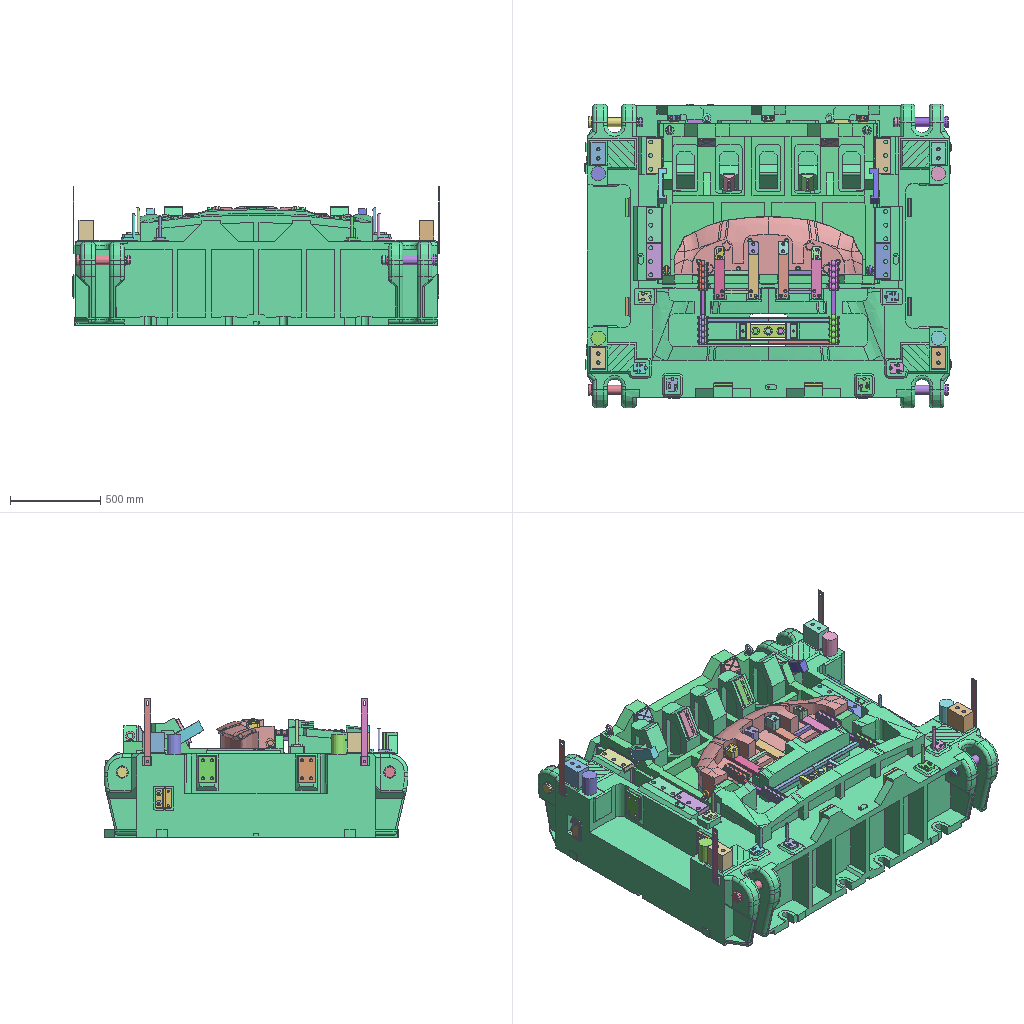Assembly | NX | 145 different items | 145 placed | box 2029 x 1680 x 765 mm
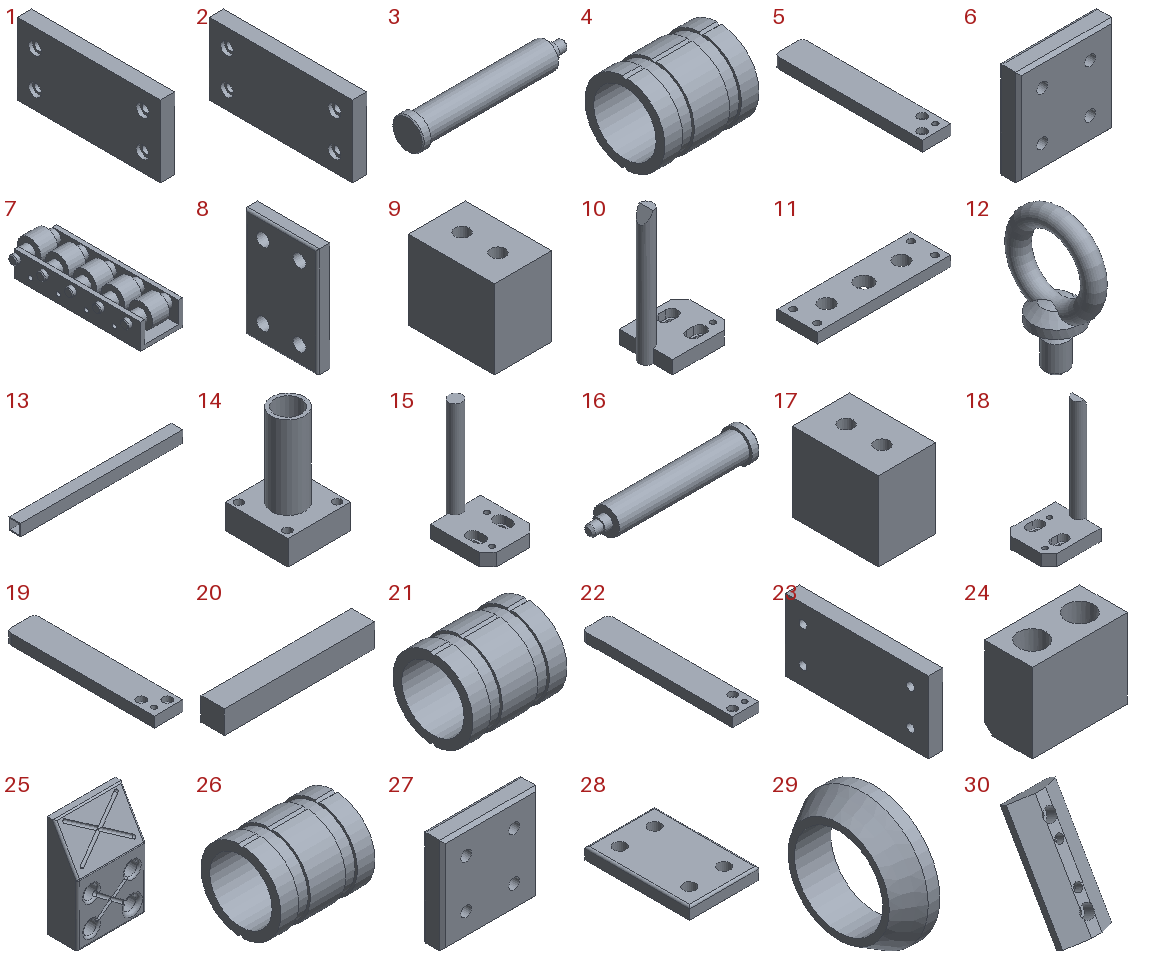Parts list (item | quantity | size | volume | features):
1 | x1 | 20 x 200 x 100 mm | 389487 mm3 | features solid 2
2 | x1 | 20 x 200 x 100 mm | 389487 mm3 | features solid 2
3 | x1 | 300 x 60 x 60 mm | 546127 mm3 | features solid 2
4 | x1 | 80 x 68 x 67.889 mm | 105275 mm3 | features solid 2
5 | x1 | 55 x 285 x 20 mm | 304183 mm3 | features solid 2
6 | x1 | 100 x 20 x 100 mm | 182887 mm3 | features solid 2
7 | x1 | 60 x 161 x 36 mm | 156058 mm3 | features solid 2
8 | x1 | 20 x 100 x 150 mm | 282244 mm3 | features solid 2
9 | x1 | 80 x 120 x 110 mm | 993294 mm3 | features solid 2
10 | x1 | 76.5 x 60 x 150 mm | 80948 mm3 | features solid 2
11 | x1 | 250 x 75 x 19 mm | 308906 mm3 | features solid 2
12 | x1 | 25 x 50 x 73 mm | 14391 mm3 | features solid 2
13 | x1 | 348.5 x 25 x 25 mm | 64124 mm3 | features solid 2
14 | x1 | 76 x 76 x 130 mm | 193450 mm3 | features solid 2
15 | x1 | 60 x 76.5 x 130 mm | 77518 mm3 | features solid 2
16 | x1 | 300 x 60 x 60 mm | 546127 mm3 | features solid 2
17 | x1 | 80 x 120 x 110 mm | 993294 mm3 | features solid 2
18 | x1 | 76.5 x 60 x 150 mm | 80948 mm3 | features solid 2
19 | x1 | 55 x 285 x 20 mm | 304183 mm3 | features solid 2
20 | x1 | 130 x 20 x 20 mm | 52000 mm3 | features solid 2
21 | x1 | 80 x 68 x 67.889 mm | 105275 mm3 | features solid 2
22 | x1 | 55 x 315 x 20 mm | 337183 mm3 | features solid 2
23 | x1 | 20 x 200 x 100 mm | 389487 mm3 | features solid 2
24 | x1 | 60 x 30 x 50 mm | 71017 mm3 | features solid 2
25 | x1 | 100 x 45 x 150 mm | 520948 mm3 | features solid 2
26 | x1 | 80 x 68 x 67.889 mm | 105275 mm3 | features solid 2
27 | x1 | 100 x 20 x 100 mm | 182887 mm3 | features solid 2
28 | x1 | 100 x 150 x 20 mm | 282244 mm3 | features solid 2
29 | x1 | 14 x 50 x 50 mm | 10965 mm3 | features solid 2
30 | x1 | 65 x 97.517 x 142.904 mm | 182247 mm3 | features solid 2
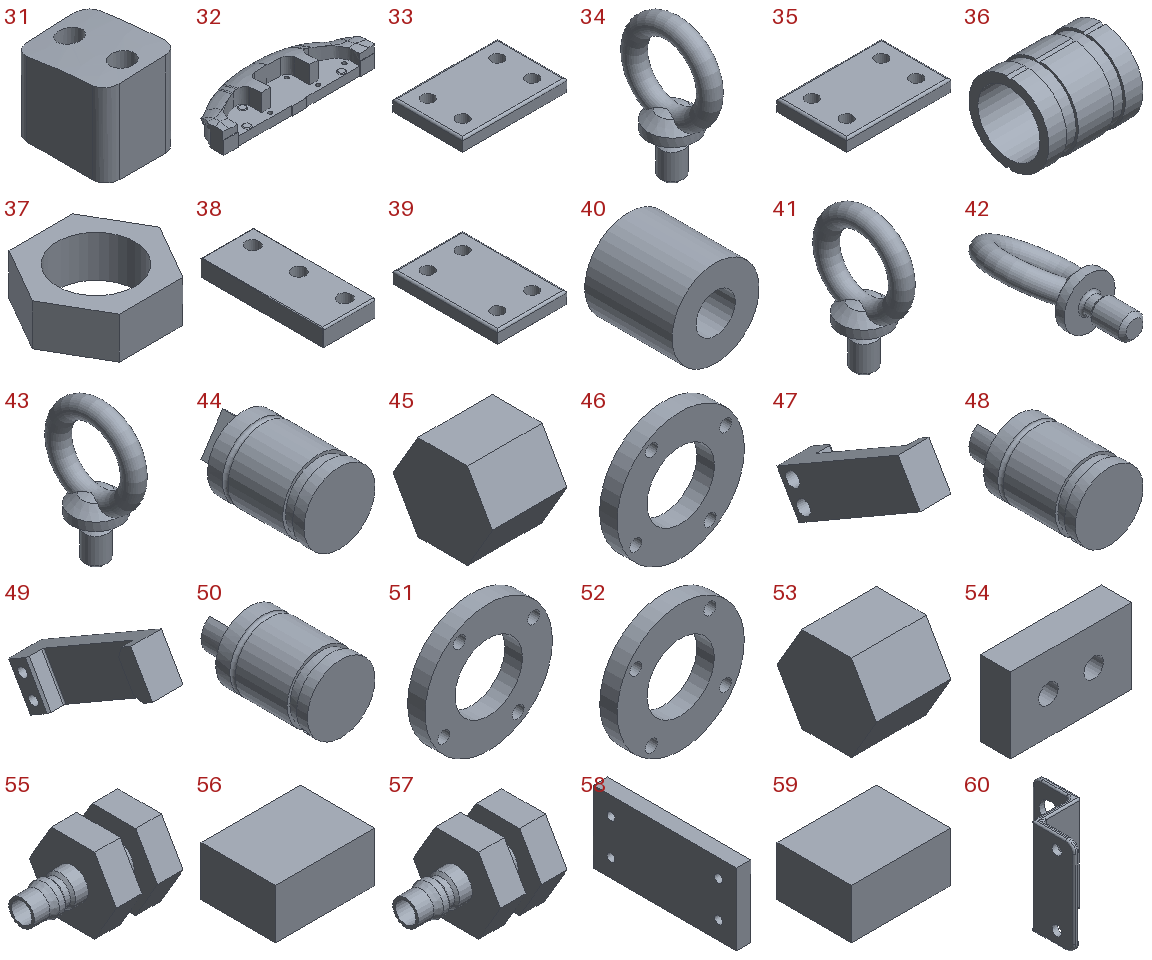31 | x1 | 55 x 70 x 64.706 mm | 206090 mm3 | features solid 2
32 | x1 | 1040 x 322.115 x 183.006 mm | 23304178 mm3 | features solid 2
33 | x1 | 150 x 100 x 20 mm | 282244 mm3 | features solid 2
34 | x1 | 25 x 50 x 73 mm | 14391 mm3 | features solid 2
35 | x1 | 150 x 100 x 20 mm | 282244 mm3 | features solid 2
36 | x1 | 80 x 68 x 67.889 mm | 105275 mm3 | features solid 2
37 | x1 | 46 x 39.837 x 15 mm | 11379 mm3 | features solid 2
38 | x1 | 85 x 200 x 28 mm | 443266 mm3 | features solid 2
39 | x1 | 100 x 150 x 20 mm | 282244 mm3 | features solid 2
40 | x1 | 40 x 40 x 40 mm | 41681 mm3 | features solid 2
41 | x1 | 25 x 50 x 73 mm | 14391 mm3 | features solid 2
42 | x1 | 43.487 x 73 x 31.878 mm | 14391 mm3 | features solid 2
43 | x1 | 25 x 50 x 73 mm | 14391 mm3 | features solid 2
44 | x1 | 50.2 x 90 x 50.2 mm | 140216 mm3 | features MAIN_BODY 2
45 | x1 | 15 x 20 x 17.321 mm | 3897 mm3 | features solid 2
46 | x1 | 95 x 13 x 95 mm | 63109 mm3 | features MAIN_BODY 2
47 | x1 | 47 x 195.411 x 147.462 mm | 335091 mm3 | features MAIN_BODY 2
48 | x1 | 50.2 x 90 x 50.2 mm | 140216 mm3 | features MAIN_BODY 2
49 | x1 | 47 x 195.411 x 147.462 mm | 335092 mm3 | features MAIN_BODY 2
50 | x1 | 50.2 x 90 x 50.2 mm | 140216 mm3 | features MAIN_BODY 2
51 | x1 | 95 x 13 x 95 mm | 63109 mm3 | features MAIN_BODY 2
52 | x1 | 95 x 13 x 95 mm | 63109 mm3 | features MAIN_BODY 2
53 | x1 | 15 x 20 x 17.321 mm | 3897 mm3 | features solid 2
54 | x1 | 80 x 20 x 50 mm | 71062 mm3 | features solid 2
55 | x1 | 50 x 34 x 29.445 mm | 18158 mm3 | features solid 2
56 | x1 | 43 x 30 x 20 mm | 24236 mm3 | features solid 2
57 | x1 | 50 x 34 x 29.445 mm | 18158 mm3 | features solid 2
58 | x1 | 20 x 200 x 100 mm | 389487 mm3 | features solid 2
59 | x1 | 43 x 30 x 20 mm | 24236 mm3 | features solid 2
60 | x1 | 51 x 93 x 110 mm | 84043 mm3 | features solid 2
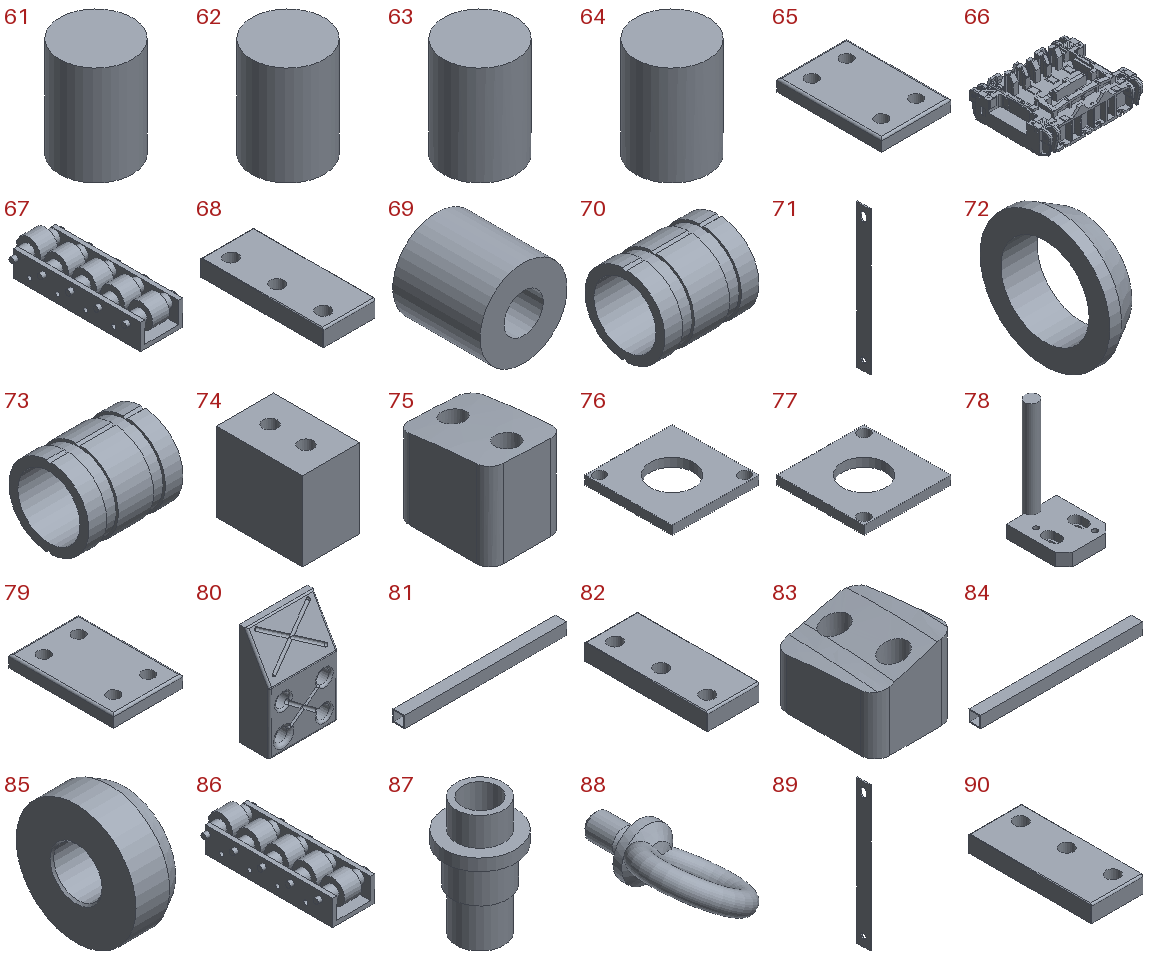61 | x1 | 80 x 80 x 120 mm | 556062 mm3 | features solid 2
62 | x1 | 80 x 80 x 120 mm | 556062 mm3 | features solid 2
63 | x1 | 80 x 80 x 120 mm | 556062 mm3 | features solid 2
64 | x1 | 80 x 80 x 120 mm | 556062 mm3 | features solid 2
65 | x1 | 100 x 150 x 20 mm | 282244 mm3 | features solid 2
66 | x1 | 2020 x 1680 x 657.116 mm | 538291554 mm3 | features solid 2
67 | x1 | 60 x 161 x 36 mm | 156058 mm3 | features solid 2
68 | x1 | 85 x 200 x 28 mm | 443266 mm3 | features solid 2
69 | x1 | 40 x 40 x 40 mm | 41681 mm3 | features solid 2
70 | x1 | 80 x 68 x 67.889 mm | 105275 mm3 | features solid 2
71 | x1 | 3 x 35 x 370 mm | 37485 mm3 | features solid 2
72 | x1 | 14 x 50 x 50 mm | 10965 mm3 | features solid 2
73 | x1 | 80 x 68 x 67.889 mm | 105275 mm3 | features solid 2
74 | x1 | 80 x 120 x 110 mm | 993294 mm3 | features solid 2
75 | x1 | 55 x 70 x 64.706 mm | 206090 mm3 | features solid 2
76 | x1 | 60 x 60 x 6 mm | 16756 mm3 | features solid 2
77 | x1 | 60 x 60 x 6 mm | 16756 mm3 | features solid 2
78 | x1 | 60 x 76.5 x 130 mm | 77518 mm3 | features solid 2
79 | x1 | 100 x 150 x 20 mm | 282244 mm3 | features solid 2
80 | x1 | 100 x 45 x 150 mm | 520948 mm3 | features solid 2
81 | x1 | 348.5 x 25 x 25 mm | 64124 mm3 | features solid 2
82 | x1 | 85 x 200 x 28 mm | 443266 mm3 | features solid 2
83 | x1 | 55 x 70 x 52.401 mm | 147496 mm3 | features solid 2
84 | x1 | 348.5 x 25 x 25 mm | 64124 mm3 | features solid 2
85 | x1 | 20 x 50 x 50 mm | 30708 mm3 | features solid 2
86 | x1 | 60 x 161 x 36 mm | 156058 mm3 | features solid 2
87 | x1 | 60 x 60 x 99 mm | 82294 mm3 | features solid 2
88 | x1 | 43.487 x 73 x 31.878 mm | 14391 mm3 | features solid 2
89 | x1 | 3 x 35 x 370 mm | 37485 mm3 | features solid 2
90 | x1 | 85 x 200 x 28 mm | 443266 mm3 | features solid 2
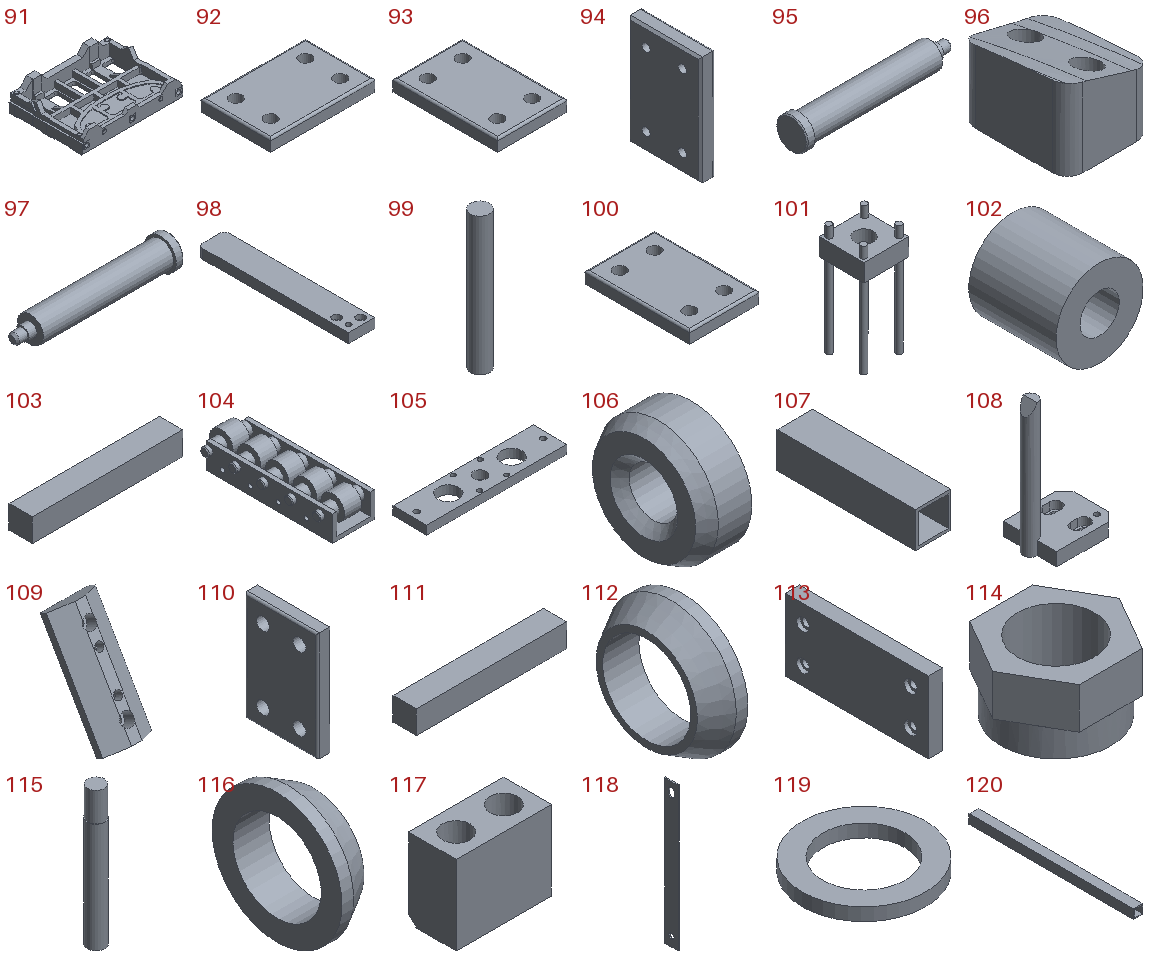91 | x1 | 1210 x 890 x 285 mm | 82458161 mm3 | features solid 2
92 | x1 | 150 x 100 x 20 mm | 282244 mm3 | features solid 2
93 | x1 | 100 x 150 x 20 mm | 282244 mm3 | features solid 2
94 | x1 | 20 x 100 x 150 mm | 282244 mm3 | features solid 2
95 | x1 | 300 x 60 x 60 mm | 546127 mm3 | features solid 2
96 | x1 | 55 x 70 x 52.401 mm | 147495 mm3 | features solid 2
97 | x1 | 300 x 60 x 60 mm | 546127 mm3 | features solid 2
98 | x1 | 55 x 315 x 20 mm | 337183 mm3 | features solid 2
99 | x1 | 32 x 32 x 235 mm | 188998 mm3 | features solid 2
100 | x1 | 100 x 150 x 20 mm | 282244 mm3 | features solid 2
101 | x1 | 76 x 76 x 189 mm | 194032 mm3 | features solid 2
102 | x1 | 40 x 40 x 40 mm | 41681 mm3 | features solid 2
103 | x1 | 130 x 20 x 20 mm | 52000 mm3 | features solid 2
104 | x1 | 60 x 161 x 36 mm | 156058 mm3 | features solid 2
105 | x1 | 310 x 75 x 19 mm | 356782 mm3 | features solid 2
106 | x1 | 20 x 50 x 50 mm | 30708 mm3 | features solid 2
107 | x1 | 25 x 97 x 25 mm | 17848 mm3 | features solid 2
108 | x1 | 76.5 x 60 x 150 mm | 80948 mm3 | features solid 2
109 | x1 | 65 x 97.517 x 142.904 mm | 182247 mm3 | features solid 2
110 | x1 | 20 x 100 x 150 mm | 282244 mm3 | features solid 2
111 | x1 | 130 x 20 x 20 mm | 52000 mm3 | features solid 2
112 | x1 | 14 x 50 x 50 mm | 10965 mm3 | features solid 2
113 | x1 | 20 x 200 x 100 mm | 389487 mm3 | features solid 2
114 | x1 | 46 x 40 x 25 mm | 17788 mm3 | features solid 2
115 | x1 | 30 x 30 x 235 mm | 161648 mm3 | features solid 2
116 | x1 | 14 x 50 x 50 mm | 10965 mm3 | features solid 2
117 | x1 | 60 x 30 x 50 mm | 71017 mm3 | features solid 2
118 | x1 | 3 x 35 x 370 mm | 37485 mm3 | features solid 2
119 | x1 | 48 x 48 x 5 mm | 5027 mm3 | features solid 2
120 | x1 | 25 x 448 x 25 mm | 82432 mm3 | features solid 2
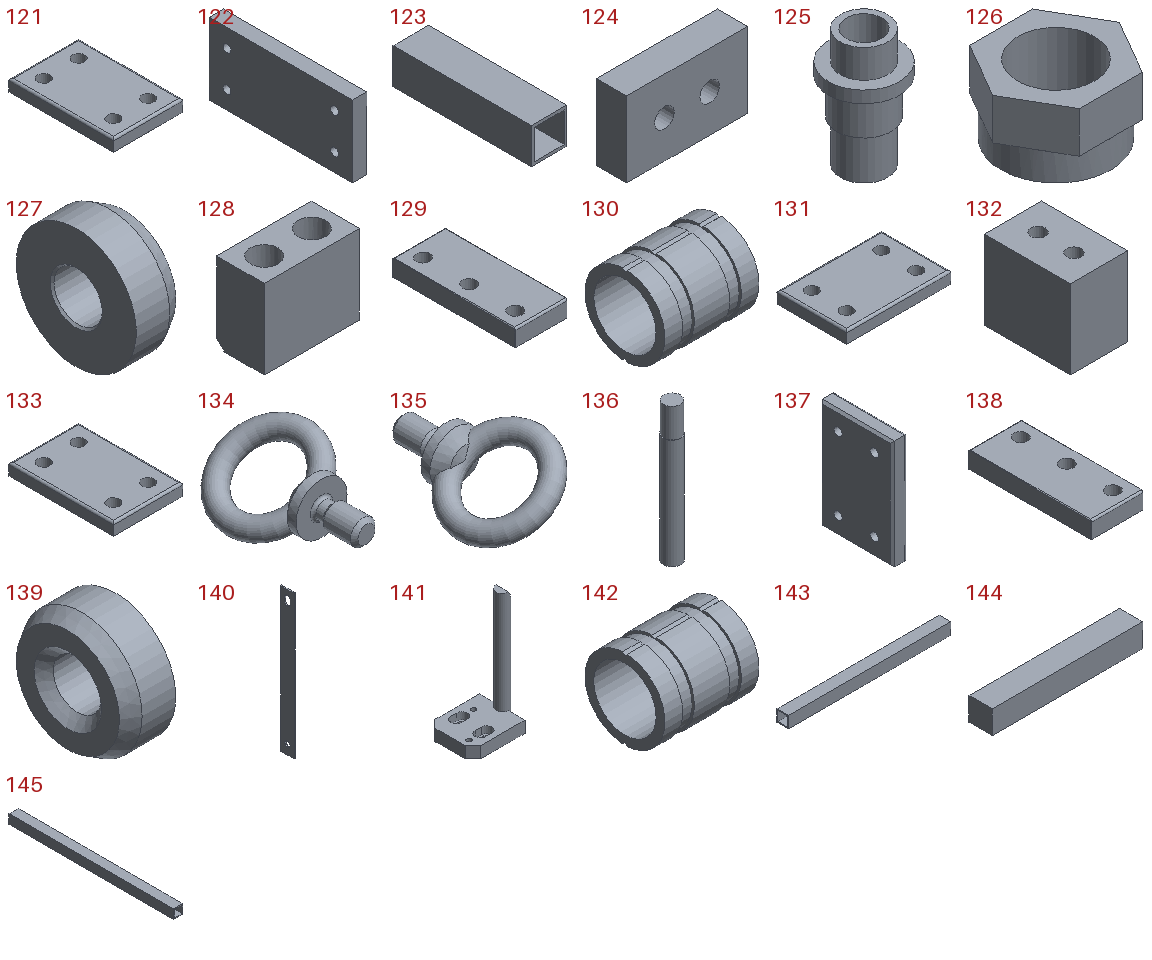121 | x1 | 100 x 150 x 20 mm | 282244 mm3 | features solid 2
122 | x1 | 20 x 200 x 100 mm | 389487 mm3 | features solid 2
123 | x1 | 25 x 97 x 25 mm | 17848 mm3 | features solid 2
124 | x1 | 80 x 20 x 50 mm | 71062 mm3 | features solid 2
125 | x1 | 60 x 60 x 99 mm | 82294 mm3 | features solid 2
126 | x1 | 46 x 40 x 25 mm | 17788 mm3 | features solid 2
127 | x1 | 20 x 50 x 50 mm | 30708 mm3 | features solid 2
128 | x1 | 60 x 30 x 50 mm | 71017 mm3 | features solid 2
129 | x1 | 85 x 200 x 28 mm | 443266 mm3 | features solid 2
130 | x1 | 80 x 68 x 67.889 mm | 105275 mm3 | features solid 2
131 | x1 | 150 x 100 x 20 mm | 282244 mm3 | features solid 2
132 | x1 | 80 x 120 x 110 mm | 993294 mm3 | features solid 2
133 | x1 | 100 x 150 x 20 mm | 282244 mm3 | features solid 2
134 | x1 | 43.487 x 73 x 31.878 mm | 14391 mm3 | features solid 2
135 | x1 | 43.487 x 73 x 31.878 mm | 14391 mm3 | features solid 2
136 | x1 | 30 x 30 x 235 mm | 161648 mm3 | features solid 2
137 | x1 | 20 x 100 x 150 mm | 282244 mm3 | features solid 2
138 | x1 | 85 x 200 x 28 mm | 443266 mm3 | features solid 2
139 | x1 | 20 x 50 x 50 mm | 30708 mm3 | features solid 2
140 | x1 | 3 x 35 x 370 mm | 37485 mm3 | features solid 2
141 | x1 | 76.5 x 60 x 150 mm | 80948 mm3 | features solid 2
142 | x1 | 80 x 68 x 67.889 mm | 105275 mm3 | features solid 2
143 | x1 | 348.5 x 25 x 25 mm | 64124 mm3 | features solid 2
144 | x1 | 130 x 20 x 20 mm | 52000 mm3 | features solid 2
145 | x1 | 25 x 448 x 25 mm | 82432 mm3 | features solid 2